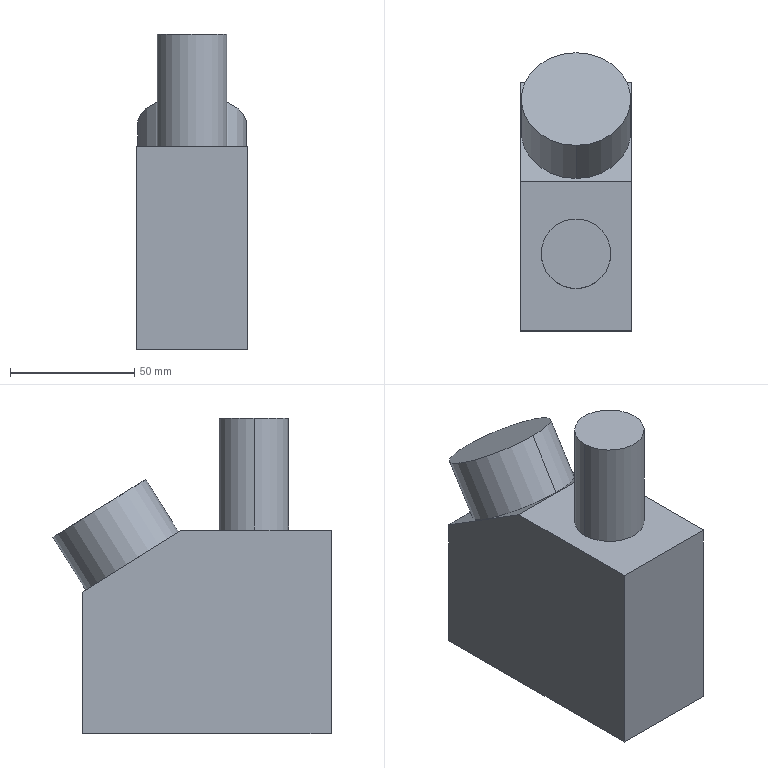Part | SolidWorks | features BaseBody 1 | 1 solid | 13 faces | box 45 x 111.906 x 127 mm | volume 412222 mm3 | plane 9 | cylinder 4 | commonest cylinder face diameters 28 x2 44 x2
STEP:
#1=CARTESIAN_POINT('',(0.,61.906,79.04));
#2=VERTEX_POINT('',#1);
#3=CARTESIAN_POINT('',(0.,24.594,102.36));
#4=VERTEX_POINT('',#3);
#5=CARTESIAN_POINT('',(0.,43.25,90.7));
#6=DIRECTION('',(0.,-0.53,-0.848));
#7=DIRECTION('',(0.,0.848,-0.53));
#8=AXIS2_PLACEMENT_3D('',#5,#6,#7);
#9=CIRCLE('',#8,22.);
#10=EDGE_CURVE('',#2,#4,#9,.T.);
#11=ORIENTED_EDGE('',*,*,#10,.F.);
#12=CARTESIAN_POINT('',(0.,43.25,90.7));
#13=DIRECTION('',(0.,-0.53,-0.848));
#14=DIRECTION('',(0.,0.848,-0.53));
#15=AXIS2_PLACEMENT_3D('',#12,#13,#14);
#16=CIRCLE('',#15,22.);
#17=EDGE_CURVE('',#4,#2,#16,.T.);
#18=ORIENTED_EDGE('',*,*,#17,.F.);
#19=EDGE_LOOP('',(#11,#18));
#20=FACE_OUTER_BOUND('',#19,.T.);
#21=CARTESIAN_POINT('',(0.,43.25,90.7));
#22=DIRECTION('',(0.,0.53,0.848));
#23=DIRECTION('',(1.,0.,0.));
#24=AXIS2_PLACEMENT_3D('',#21,#22,#23);
#25=PLANE('',#24);
#26=ADVANCED_FACE('',(#20),#25,.T.);
#27=CARTESIAN_POINT('',(-14.,-19.,127.));
#28=VERTEX_POINT('',#27);
#29=CARTESIAN_POINT('',(14.,-19.,127.));
#30=VERTEX_POINT('',#29);
#31=CARTESIAN_POINT('',(0.,-19.,127.));
#32=DIRECTION('',(0.,0.,-1.));
#33=DIRECTION('',(-1.,0.,0.));
#34=AXIS2_PLACEMENT_3D('',#31,#32,#33);
#35=CIRCLE('',#34,14.);
#36=EDGE_CURVE('',#28,#30,#35,.T.);
#37=ORIENTED_EDGE('',*,*,#36,.F.);
#38=CARTESIAN_POINT('',(0.,-19.,127.));
#39=DIRECTION('',(0.,0.,-1.));
#40=DIRECTION('',(-1.,0.,0.));
#41=AXIS2_PLACEMENT_3D('',#38,#39,#40);
#42=CIRCLE('',#41,14.);
#43=EDGE_CURVE('',#30,#28,#42,.T.);
#44=ORIENTED_EDGE('',*,*,#43,.F.);
#45=EDGE_LOOP('',(#37,#44));
#46=FACE_OUTER_BOUND('',#45,.T.);
#47=CARTESIAN_POINT('',(0.,-19.,127.));
#48=DIRECTION('',(0.,0.,1.));
#49=DIRECTION('',(1.,0.,0.));
#50=AXIS2_PLACEMENT_3D('',#47,#48,#49);
#51=PLANE('',#50);
#52=ADVANCED_FACE('',(#46),#51,.T.);
#53=CARTESIAN_POINT('',(0.,11.344,81.16));
#54=VERTEX_POINT('',#53);
#55=CARTESIAN_POINT('',(0.,24.594,102.36));
#56=DIRECTION('',(0.,-0.53,-0.848));
#57=VECTOR('',#56,1000.);
#58=LINE('',#55,#57);
#59=EDGE_CURVE('',#4,#54,#58,.T.);
#60=ORIENTED_EDGE('',*,*,#59,.F.);
#61=ORIENTED_EDGE('',*,*,#17,.T.);
#62=CARTESIAN_POINT('',(0.,48.656,57.84));
#63=VERTEX_POINT('',#62);
#64=CARTESIAN_POINT('',(0.,61.906,79.04));
#65=DIRECTION('',(0.,-0.53,-0.848));
#66=VECTOR('',#65,1000.);
#67=LINE('',#64,#66);
#68=EDGE_CURVE('',#2,#63,#67,.T.);
#69=ORIENTED_EDGE('',*,*,#68,.T.);
#70=CARTESIAN_POINT('',(0.,30.,69.5));
#71=DIRECTION('',(0.,-0.53,-0.848));
#72=DIRECTION('',(0.,0.848,-0.53));
#73=AXIS2_PLACEMENT_3D('',#70,#71,#72);
#74=CIRCLE('',#73,22.);
#75=EDGE_CURVE('',#54,#63,#74,.T.);
#76=ORIENTED_EDGE('',*,*,#75,.F.);
#77=EDGE_LOOP('',(#60,#61,#69,#76));
#78=FACE_OUTER_BOUND('',#77,.T.);
#79=CARTESIAN_POINT('',(0.,43.25,90.7));
#80=DIRECTION('',(0.,-0.53,-0.848));
#81=DIRECTION('',(0.,0.848,-0.53));
#82=AXIS2_PLACEMENT_3D('',#79,#80,#81);
#83=CYLINDRICAL_SURFACE('',#82,22.);
#84=ADVANCED_FACE('',(#78),#83,.T.);
#85=CARTESIAN_POINT('',(14.,-19.,82.));
#86=VERTEX_POINT('',#85);
#87=CARTESIAN_POINT('',(14.,-19.,127.));
#88=DIRECTION('',(0.,0.,-1.));
#89=VECTOR('',#88,1000.);
#90=LINE('',#87,#89);
#91=EDGE_CURVE('',#30,#86,#90,.T.);
#92=ORIENTED_EDGE('',*,*,#91,.F.);
#93=ORIENTED_EDGE('',*,*,#43,.T.);
#94=CARTESIAN_POINT('',(-14.,-19.,82.));
#95=VERTEX_POINT('',#94);
#96=CARTESIAN_POINT('',(-14.,-19.,127.));
#97=DIRECTION('',(0.,0.,-1.));
#98=VECTOR('',#97,1000.);
#99=LINE('',#96,#98);
#100=EDGE_CURVE('',#28,#95,#99,.T.);
#101=ORIENTED_EDGE('',*,*,#100,.T.);
#102=CARTESIAN_POINT('',(0.,-19.,82.));
#103=DIRECTION('',(0.,0.,-1.));
#104=DIRECTION('',(-1.,0.,0.));
#105=AXIS2_PLACEMENT_3D('',#102,#103,#104);
#106=CIRCLE('',#105,14.);
#107=EDGE_CURVE('',#86,#95,#106,.T.);
#108=ORIENTED_EDGE('',*,*,#107,.F.);
#109=EDGE_LOOP('',(#92,#93,#101,#108));
#110=FACE_OUTER_BOUND('',#109,.T.);
#111=CARTESIAN_POINT('',(0.,-19.,127.));
#112=DIRECTION('',(0.,0.,-1.));
#113=DIRECTION('',(-1.,0.,0.));
#114=AXIS2_PLACEMENT_3D('',#111,#112,#113);
#115=CYLINDRICAL_SURFACE('',#114,14.);
#116=ADVANCED_FACE('',(#110),#115,.T.);
#117=CARTESIAN_POINT('',(22.5,10.,82.));
#118=VERTEX_POINT('',#117);
#119=CARTESIAN_POINT('',(22.5,50.,57.));
#120=VERTEX_POINT('',#119);
#121=CARTESIAN_POINT('',(22.5,10.,82.));
#122=DIRECTION('',(0.,0.848,-0.53));
#123=VECTOR('',#122,1000.);
#124=LINE('',#121,#123);
#125=EDGE_CURVE('',#118,#120,#124,.T.);
#126=ORIENTED_EDGE('',*,*,#125,.F.);
#127=CARTESIAN_POINT('',(22.5,-50.,82.));
#128=VERTEX_POINT('',#127);
#129=CARTESIAN_POINT('',(22.5,0.,82.));
#130=DIRECTION('',(0.,1.,0.));
#131=VECTOR('',#130,1000.);
#132=LINE('',#129,#131);
#133=EDGE_CURVE('',#128,#118,#132,.T.);
#134=ORIENTED_EDGE('',*,*,#133,.F.);
#135=CARTESIAN_POINT('',(22.5,-50.,0.));
#136=VERTEX_POINT('',#135);
#137=CARTESIAN_POINT('',(22.5,-50.,82.));
#138=DIRECTION('',(0.,0.,-1.));
#139=VECTOR('',#138,1000.);
#140=LINE('',#137,#139);
#141=EDGE_CURVE('',#128,#136,#140,.T.);
#142=ORIENTED_EDGE('',*,*,#141,.T.);
#143=CARTESIAN_POINT('',(22.5,50.,0.));
#144=VERTEX_POINT('',#143);
#145=CARTESIAN_POINT('',(22.5,0.,0.));
#146=DIRECTION('',(0.,1.,0.));
#147=VECTOR('',#146,1000.);
#148=LINE('',#145,#147);
#149=EDGE_CURVE('',#136,#144,#148,.T.);
#150=ORIENTED_EDGE('',*,*,#149,.T.);
#151=CARTESIAN_POINT('',(22.5,50.,82.));
#152=DIRECTION('',(0.,0.,1.));
#153=VECTOR('',#152,1000.);
#154=LINE('',#151,#153);
#155=EDGE_CURVE('',#144,#120,#154,.T.);
#156=ORIENTED_EDGE('',*,*,#155,.T.);
#157=EDGE_LOOP('',(#126,#134,#142,#150,#156));
#158=FACE_OUTER_BOUND('',#157,.T.);
#159=CARTESIAN_POINT('',(22.5,50.,82.));
#160=DIRECTION('',(-1.,0.,0.));
#161=DIRECTION('',(0.,1.,0.));
#162=AXIS2_PLACEMENT_3D('',#159,#160,#161);
#163=PLANE('',#162);
#164=ADVANCED_FACE('',(#158),#163,.F.);
#165=ORIENTED_EDGE('',*,*,#141,.F.);
#166=CARTESIAN_POINT('',(-22.5,-50.,82.));
#167=VERTEX_POINT('',#166);
#168=CARTESIAN_POINT('',(0.,-50.,82.));
#169=DIRECTION('',(1.,0.,0.));
#170=VECTOR('',#169,1000.);
#171=LINE('',#168,#170);
#172=EDGE_CURVE('',#167,#128,#171,.T.);
#173=ORIENTED_EDGE('',*,*,#172,.F.);
#174=CARTESIAN_POINT('',(-22.5,-50.,0.));
#175=VERTEX_POINT('',#174);
#176=CARTESIAN_POINT('',(-22.5,-50.,82.));
#177=DIRECTION('',(0.,0.,-1.));
#178=VECTOR('',#177,1000.);
#179=LINE('',#176,#178);
#180=EDGE_CURVE('',#167,#175,#179,.T.);
#181=ORIENTED_EDGE('',*,*,#180,.T.);
#182=CARTESIAN_POINT('',(0.,-50.,0.));
#183=DIRECTION('',(1.,0.,0.));
#184=VECTOR('',#183,1000.);
#185=LINE('',#182,#184);
#186=EDGE_CURVE('',#175,#136,#185,.T.);
#187=ORIENTED_EDGE('',*,*,#186,.T.);
#188=EDGE_LOOP('',(#165,#173,#181,#187));
#189=FACE_OUTER_BOUND('',#188,.T.);
#190=CARTESIAN_POINT('',(-22.5,-50.,82.));
#191=DIRECTION('',(0.,1.,0.));
#192=DIRECTION('',(1.,0.,0.));
#193=AXIS2_PLACEMENT_3D('',#190,#191,#192);
#194=PLANE('',#193);
#195=ADVANCED_FACE('',(#189),#194,.F.);
#196=ORIENTED_EDGE('',*,*,#186,.F.);
#197=CARTESIAN_POINT('',(-22.5,50.,0.));
#198=VERTEX_POINT('',#197);
#199=CARTESIAN_POINT('',(-22.5,50.,0.));
#200=DIRECTION('',(0.,1.,0.));
#201=VECTOR('',#200,1000.);
#202=LINE('',#199,#201);
#203=EDGE_CURVE('',#175,#198,#202,.T.);
#204=ORIENTED_EDGE('',*,*,#203,.T.);
#205=CARTESIAN_POINT('',(-22.5,50.,0.));
#206=DIRECTION('',(1.,0.,0.));
#207=VECTOR('',#206,1000.);
#208=LINE('',#205,#207);
#209=EDGE_CURVE('',#198,#144,#208,.T.);
#210=ORIENTED_EDGE('',*,*,#209,.T.);
#211=ORIENTED_EDGE('',*,*,#149,.F.);
#212=EDGE_LOOP('',(#196,#204,#210,#211));
#213=FACE_OUTER_BOUND('',#212,.T.);
#214=CARTESIAN_POINT('',(0.,0.,0.));
#215=DIRECTION('',(0.,0.,1.));
#216=DIRECTION('',(1.,0.,0.));
#217=AXIS2_PLACEMENT_3D('',#214,#215,#216);
#218=PLANE('',#217);
#219=ADVANCED_FACE('',(#213),#218,.F.);
#220=CARTESIAN_POINT('',(-22.5,50.,57.));
#221=VERTEX_POINT('',#220);
#222=CARTESIAN_POINT('',(0.,50.,57.));
#223=DIRECTION('',(-1.,0.,0.));
#224=VECTOR('',#223,1000.);
#225=LINE('',#222,#224);
#226=EDGE_CURVE('',#120,#221,#225,.T.);
#227=ORIENTED_EDGE('',*,*,#226,.F.);
#228=ORIENTED_EDGE('',*,*,#155,.F.);
#229=ORIENTED_EDGE('',*,*,#209,.F.);
#230=CARTESIAN_POINT('',(-22.5,50.,82.));
#231=DIRECTION('',(0.,0.,1.));
#232=VECTOR('',#231,1000.);
#233=LINE('',#230,#232);
#234=EDGE_CURVE('',#198,#221,#233,.T.);
#235=ORIENTED_EDGE('',*,*,#234,.T.);
#236=EDGE_LOOP('',(#227,#228,#229,#235));
#237=FACE_OUTER_BOUND('',#236,.T.);
#238=CARTESIAN_POINT('',(-22.5,50.,82.));
#239=DIRECTION('',(0.,-1.,0.));
#240=DIRECTION('',(-1.,0.,0.));
#241=AXIS2_PLACEMENT_3D('',#238,#239,#240);
#242=PLANE('',#241);
#243=ADVANCED_FACE('',(#237),#242,.F.);
#244=CARTESIAN_POINT('',(0.,30.,69.5));
#245=DIRECTION('',(0.,-0.53,-0.848));
#246=DIRECTION('',(0.,0.848,-0.53));
#247=AXIS2_PLACEMENT_3D('',#244,#245,#246);
#248=CIRCLE('',#247,22.);
#249=EDGE_CURVE('',#63,#54,#248,.T.);
#250=ORIENTED_EDGE('',*,*,#249,.T.);
#251=ORIENTED_EDGE('',*,*,#75,.T.);
#252=EDGE_LOOP('',(#250,#251));
#253=FACE_BOUND('',#252,.T.);
#254=CARTESIAN_POINT('',(-22.5,10.,82.));
#255=VERTEX_POINT('',#254);
#256=CARTESIAN_POINT('',(-22.5,50.,57.));
#257=DIRECTION('',(0.,-0.848,0.53));
#258=VECTOR('',#257,1000.);
#259=LINE('',#256,#258);
#260=EDGE_CURVE('',#221,#255,#259,.T.);
#261=ORIENTED_EDGE('',*,*,#260,.T.);
#262=CARTESIAN_POINT('',(0.,10.,82.));
#263=DIRECTION('',(-1.,0.,0.));
#264=VECTOR('',#263,1000.);
#265=LINE('',#262,#264);
#266=EDGE_CURVE('',#118,#255,#265,.T.);
#267=ORIENTED_EDGE('',*,*,#266,.F.);
#268=ORIENTED_EDGE('',*,*,#125,.T.);
#269=ORIENTED_EDGE('',*,*,#226,.T.);
#270=EDGE_LOOP('',(#261,#267,#268,#269));
#271=FACE_OUTER_BOUND('',#270,.T.);
#272=CARTESIAN_POINT('',(0.,10.,82.));
#273=DIRECTION('',(0.,0.53,0.848));
#274=DIRECTION('',(1.,0.,0.));
#275=AXIS2_PLACEMENT_3D('',#272,#273,#274);
#276=PLANE('',#275);
#277=ADVANCED_FACE('',(#253,#271),#276,.T.);
#278=CARTESIAN_POINT('',(0.,-19.,82.));
#279=DIRECTION('',(0.,0.,-1.));
#280=DIRECTION('',(-1.,0.,0.));
#281=AXIS2_PLACEMENT_3D('',#278,#279,#280);
#282=CIRCLE('',#281,14.);
#283=EDGE_CURVE('',#95,#86,#282,.T.);
#284=ORIENTED_EDGE('',*,*,#283,.T.);
#285=ORIENTED_EDGE('',*,*,#107,.T.);
#286=EDGE_LOOP('',(#284,#285));
#287=FACE_BOUND('',#286,.T.);
#288=CARTESIAN_POINT('',(-22.5,50.,82.));
#289=DIRECTION('',(0.,-1.,0.));
#290=VECTOR('',#289,1000.);
#291=LINE('',#288,#290);
#292=EDGE_CURVE('',#255,#167,#291,.T.);
#293=ORIENTED_EDGE('',*,*,#292,.T.);
#294=ORIENTED_EDGE('',*,*,#172,.T.);
#295=ORIENTED_EDGE('',*,*,#133,.T.);
#296=ORIENTED_EDGE('',*,*,#266,.T.);
#297=EDGE_LOOP('',(#293,#294,#295,#296));
#298=FACE_OUTER_BOUND('',#297,.T.);
#299=CARTESIAN_POINT('',(0.,0.,82.));
#300=DIRECTION('',(0.,0.,1.));
#301=DIRECTION('',(1.,0.,0.));
#302=AXIS2_PLACEMENT_3D('',#299,#300,#301);
#303=PLANE('',#302);
#304=ADVANCED_FACE('',(#287,#298),#303,.T.);
#305=ORIENTED_EDGE('',*,*,#260,.F.);
#306=ORIENTED_EDGE('',*,*,#234,.F.);
#307=ORIENTED_EDGE('',*,*,#203,.F.);
#308=ORIENTED_EDGE('',*,*,#180,.F.);
#309=ORIENTED_EDGE('',*,*,#292,.F.);
#310=EDGE_LOOP('',(#305,#306,#307,#308,#309));
#311=FACE_OUTER_BOUND('',#310,.T.);
#312=CARTESIAN_POINT('',(-22.5,50.,82.));
#313=DIRECTION('',(1.,0.,0.));
#314=DIRECTION('',(0.,1.,0.));
#315=AXIS2_PLACEMENT_3D('',#312,#313,#314);
#316=PLANE('',#315);
#317=ADVANCED_FACE('',(#311),#316,.F.);
#318=ORIENTED_EDGE('',*,*,#10,.T.);
#319=ORIENTED_EDGE('',*,*,#59,.T.);
#320=ORIENTED_EDGE('',*,*,#249,.F.);
#321=ORIENTED_EDGE('',*,*,#68,.F.);
#322=EDGE_LOOP('',(#318,#319,#320,#321));
#323=FACE_OUTER_BOUND('',#322,.T.);
#324=CARTESIAN_POINT('',(0.,43.25,90.7));
#325=DIRECTION('',(0.,-0.53,-0.848));
#326=DIRECTION('',(0.,0.848,-0.53));
#327=AXIS2_PLACEMENT_3D('',#324,#325,#326);
#328=CYLINDRICAL_SURFACE('',#327,22.);
#329=ADVANCED_FACE('',(#323),#328,.T.);
#330=ORIENTED_EDGE('',*,*,#36,.T.);
#331=ORIENTED_EDGE('',*,*,#91,.T.);
#332=ORIENTED_EDGE('',*,*,#283,.F.);
#333=ORIENTED_EDGE('',*,*,#100,.F.);
#334=EDGE_LOOP('',(#330,#331,#332,#333));
#335=FACE_OUTER_BOUND('',#334,.T.);
#336=CARTESIAN_POINT('',(0.,-19.,127.));
#337=DIRECTION('',(0.,0.,-1.));
#338=DIRECTION('',(-1.,0.,0.));
#339=AXIS2_PLACEMENT_3D('',#336,#337,#338);
#340=CYLINDRICAL_SURFACE('',#339,14.);
#341=ADVANCED_FACE('',(#335),#340,.T.);
#342=CLOSED_SHELL('',(#26,#52,#84,#116,#164,#195,#219,#243,#277,#304,#317,#329,#341));
#343=MANIFOLD_SOLID_BREP('',#342);
#344=CARTESIAN_POINT('',(0.,0.,0.));
#345=DIRECTION('',(0.,0.,1.));
#346=DIRECTION('',(1.,0.,0.));
#347=AXIS2_PLACEMENT_3D('',#344,#345,#346);
#348=(LENGTH_UNIT()NAMED_UNIT(*)SI_UNIT(.MILLI.,.METRE.));
#349=UNCERTAINTY_MEASURE_WITH_UNIT(LENGTH_MEASURE(0.00001),#348,'','');
#350=(NAMED_UNIT(*)PLANE_ANGLE_UNIT()SI_UNIT($,.RADIAN.));
#351=(NAMED_UNIT(*)SI_UNIT($,.STERADIAN.)SOLID_ANGLE_UNIT());
#352=(GEOMETRIC_REPRESENTATION_CONTEXT(3)GLOBAL_UNCERTAINTY_ASSIGNED_CONTEXT((#349))GLOBAL_UNIT_ASSIGNED_CONTEXT((#348,#350,#351))REPRESENTATION_CONTEXT('',''));
#353=ADVANCED_BREP_SHAPE_REPRESENTATION('',(#343,#347),#352);